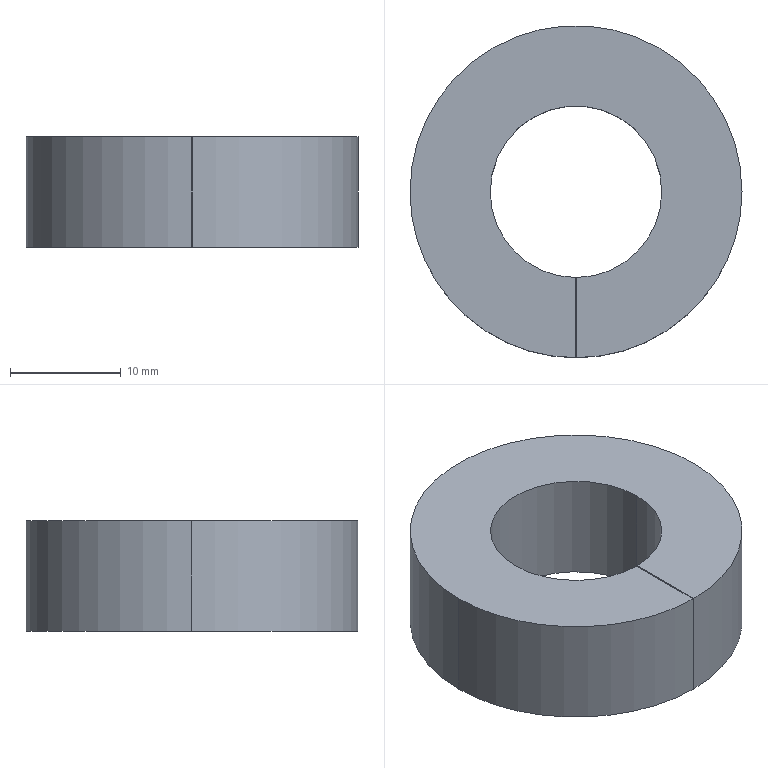Part | SolidWorks | features Extrusion 1, ICE 1 | 1 solid | 10 faces | box 30 x 30 x 10 mm | volume 5174 mm3 | cylinder 6 | plane 4 | commonest cylinder face diameters 15.5 x3 30 x3
STEP:
#1=CARTESIAN_POINT('',(0.05,-7.75,10.));
#2=VERTEX_POINT('',#1);
#3=CARTESIAN_POINT('',(7.75,0.,10.));
#4=VERTEX_POINT('',#3);
#5=CARTESIAN_POINT('',(0.,0.,10.));
#6=DIRECTION('',(0.,0.,1.));
#7=DIRECTION('',(1.,0.,0.));
#8=AXIS2_PLACEMENT_3D('',#5,#6,#7);
#9=CIRCLE('',#8,7.75);
#10=EDGE_CURVE('',#2,#4,#9,.T.);
#11=ORIENTED_EDGE('',*,*,#10,.T.);
#12=CARTESIAN_POINT('',(7.75,0.,0.));
#13=VERTEX_POINT('',#12);
#14=CARTESIAN_POINT('',(7.75,0.,10.));
#15=DIRECTION('',(0.,0.,-1.));
#16=VECTOR('',#15,1000.);
#17=LINE('',#14,#16);
#18=EDGE_CURVE('',#4,#13,#17,.T.);
#19=ORIENTED_EDGE('',*,*,#18,.T.);
#20=CARTESIAN_POINT('',(0.05,-7.75,0.));
#21=VERTEX_POINT('',#20);
#22=CARTESIAN_POINT('',(0.,0.,0.));
#23=DIRECTION('',(0.,0.,1.));
#24=DIRECTION('',(1.,0.,0.));
#25=AXIS2_PLACEMENT_3D('',#22,#23,#24);
#26=CIRCLE('',#25,7.75);
#27=EDGE_CURVE('',#21,#13,#26,.T.);
#28=ORIENTED_EDGE('',*,*,#27,.F.);
#29=CARTESIAN_POINT('',(0.05,-7.75,10.));
#30=DIRECTION('',(0.,0.,-1.));
#31=VECTOR('',#30,1000.);
#32=LINE('',#29,#31);
#33=EDGE_CURVE('',#2,#21,#32,.T.);
#34=ORIENTED_EDGE('',*,*,#33,.F.);
#35=EDGE_LOOP('',(#11,#19,#28,#34));
#36=FACE_OUTER_BOUND('',#35,.T.);
#37=CARTESIAN_POINT('',(0.,0.,10.));
#38=DIRECTION('',(0.,0.,-1.));
#39=DIRECTION('',(-1.,0.,0.));
#40=AXIS2_PLACEMENT_3D('',#37,#38,#39);
#41=CYLINDRICAL_SURFACE('',#40,7.75);
#42=ADVANCED_FACE('',(#36),#41,.F.);
#43=ORIENTED_EDGE('',*,*,#18,.F.);
#44=CARTESIAN_POINT('',(-7.75,0.,10.));
#45=VERTEX_POINT('',#44);
#46=CARTESIAN_POINT('',(0.,0.,10.));
#47=DIRECTION('',(0.,0.,1.));
#48=DIRECTION('',(1.,0.,0.));
#49=AXIS2_PLACEMENT_3D('',#46,#47,#48);
#50=CIRCLE('',#49,7.75);
#51=EDGE_CURVE('',#4,#45,#50,.T.);
#52=ORIENTED_EDGE('',*,*,#51,.T.);
#53=CARTESIAN_POINT('',(-7.75,0.,0.));
#54=VERTEX_POINT('',#53);
#55=CARTESIAN_POINT('',(-7.75,0.,10.));
#56=DIRECTION('',(0.,0.,-1.));
#57=VECTOR('',#56,1000.);
#58=LINE('',#55,#57);
#59=EDGE_CURVE('',#45,#54,#58,.T.);
#60=ORIENTED_EDGE('',*,*,#59,.T.);
#61=CARTESIAN_POINT('',(0.,0.,0.));
#62=DIRECTION('',(0.,0.,1.));
#63=DIRECTION('',(1.,0.,0.));
#64=AXIS2_PLACEMENT_3D('',#61,#62,#63);
#65=CIRCLE('',#64,7.75);
#66=EDGE_CURVE('',#13,#54,#65,.T.);
#67=ORIENTED_EDGE('',*,*,#66,.F.);
#68=EDGE_LOOP('',(#43,#52,#60,#67));
#69=FACE_OUTER_BOUND('',#68,.T.);
#70=CARTESIAN_POINT('',(0.,0.,10.));
#71=DIRECTION('',(0.,0.,-1.));
#72=DIRECTION('',(-1.,0.,0.));
#73=AXIS2_PLACEMENT_3D('',#70,#71,#72);
#74=CYLINDRICAL_SURFACE('',#73,7.75);
#75=ADVANCED_FACE('',(#69),#74,.F.);
#76=CARTESIAN_POINT('',(15.,0.,10.));
#77=VERTEX_POINT('',#76);
#78=CARTESIAN_POINT('',(-15.,0.,10.));
#79=VERTEX_POINT('',#78);
#80=CARTESIAN_POINT('',(0.,0.,10.));
#81=DIRECTION('',(0.,0.,1.));
#82=DIRECTION('',(1.,0.,0.));
#83=AXIS2_PLACEMENT_3D('',#80,#81,#82);
#84=CIRCLE('',#83,15.);
#85=EDGE_CURVE('',#77,#79,#84,.T.);
#86=ORIENTED_EDGE('',*,*,#85,.F.);
#87=CARTESIAN_POINT('',(15.,0.,0.));
#88=VERTEX_POINT('',#87);
#89=CARTESIAN_POINT('',(15.,0.,10.));
#90=DIRECTION('',(0.,0.,-1.));
#91=VECTOR('',#90,1000.);
#92=LINE('',#89,#91);
#93=EDGE_CURVE('',#77,#88,#92,.T.);
#94=ORIENTED_EDGE('',*,*,#93,.T.);
#95=CARTESIAN_POINT('',(-15.,0.,0.));
#96=VERTEX_POINT('',#95);
#97=CARTESIAN_POINT('',(0.,0.,0.));
#98=DIRECTION('',(0.,0.,1.));
#99=DIRECTION('',(1.,0.,0.));
#100=AXIS2_PLACEMENT_3D('',#97,#98,#99);
#101=CIRCLE('',#100,15.);
#102=EDGE_CURVE('',#88,#96,#101,.T.);
#103=ORIENTED_EDGE('',*,*,#102,.T.);
#104=CARTESIAN_POINT('',(-15.,0.,10.));
#105=DIRECTION('',(0.,0.,-1.));
#106=VECTOR('',#105,1000.);
#107=LINE('',#104,#106);
#108=EDGE_CURVE('',#79,#96,#107,.T.);
#109=ORIENTED_EDGE('',*,*,#108,.F.);
#110=EDGE_LOOP('',(#86,#94,#103,#109));
#111=FACE_OUTER_BOUND('',#110,.T.);
#112=CARTESIAN_POINT('',(0.,0.,10.));
#113=DIRECTION('',(0.,0.,-1.));
#114=DIRECTION('',(-1.,0.,0.));
#115=AXIS2_PLACEMENT_3D('',#112,#113,#114);
#116=CYLINDRICAL_SURFACE('',#115,15.);
#117=ADVANCED_FACE('',(#111),#116,.T.);
#118=CARTESIAN_POINT('',(-0.05,-15.,10.));
#119=VERTEX_POINT('',#118);
#120=CARTESIAN_POINT('',(0.,0.,10.));
#121=DIRECTION('',(0.,0.,1.));
#122=DIRECTION('',(1.,0.,0.));
#123=AXIS2_PLACEMENT_3D('',#120,#121,#122);
#124=CIRCLE('',#123,15.);
#125=EDGE_CURVE('',#79,#119,#124,.T.);
#126=ORIENTED_EDGE('',*,*,#125,.F.);
#127=ORIENTED_EDGE('',*,*,#108,.T.);
#128=CARTESIAN_POINT('',(-0.05,-15.,0.));
#129=VERTEX_POINT('',#128);
#130=CARTESIAN_POINT('',(0.,0.,0.));
#131=DIRECTION('',(0.,0.,1.));
#132=DIRECTION('',(1.,0.,0.));
#133=AXIS2_PLACEMENT_3D('',#130,#131,#132);
#134=CIRCLE('',#133,15.);
#135=EDGE_CURVE('',#96,#129,#134,.T.);
#136=ORIENTED_EDGE('',*,*,#135,.T.);
#137=CARTESIAN_POINT('',(-0.05,-15.,10.));
#138=DIRECTION('',(0.,0.,1.));
#139=VECTOR('',#138,1000.);
#140=LINE('',#137,#139);
#141=EDGE_CURVE('',#129,#119,#140,.T.);
#142=ORIENTED_EDGE('',*,*,#141,.T.);
#143=EDGE_LOOP('',(#126,#127,#136,#142));
#144=FACE_OUTER_BOUND('',#143,.T.);
#145=CARTESIAN_POINT('',(0.,0.,10.));
#146=DIRECTION('',(0.,0.,-1.));
#147=DIRECTION('',(-1.,0.,0.));
#148=AXIS2_PLACEMENT_3D('',#145,#146,#147);
#149=CYLINDRICAL_SURFACE('',#148,15.);
#150=ADVANCED_FACE('',(#144),#149,.T.);
#151=CARTESIAN_POINT('',(0.05,-15.,10.));
#152=VERTEX_POINT('',#151);
#153=CARTESIAN_POINT('',(0.05,3.484,10.));
#154=DIRECTION('',(0.,1.,0.));
#155=VECTOR('',#154,1000.);
#156=LINE('',#153,#155);
#157=EDGE_CURVE('',#152,#2,#156,.T.);
#158=ORIENTED_EDGE('',*,*,#157,.F.);
#159=CARTESIAN_POINT('',(0.,0.,10.));
#160=DIRECTION('',(0.,0.,1.));
#161=DIRECTION('',(1.,0.,0.));
#162=AXIS2_PLACEMENT_3D('',#159,#160,#161);
#163=CIRCLE('',#162,15.);
#164=EDGE_CURVE('',#152,#77,#163,.T.);
#165=ORIENTED_EDGE('',*,*,#164,.T.);
#166=ORIENTED_EDGE('',*,*,#85,.T.);
#167=ORIENTED_EDGE('',*,*,#125,.T.);
#168=CARTESIAN_POINT('',(-0.05,-7.75,10.));
#169=VERTEX_POINT('',#168);
#170=CARTESIAN_POINT('',(-0.05,3.484,10.));
#171=DIRECTION('',(0.,-1.,0.));
#172=VECTOR('',#171,1000.);
#173=LINE('',#170,#172);
#174=EDGE_CURVE('',#169,#119,#173,.T.);
#175=ORIENTED_EDGE('',*,*,#174,.F.);
#176=CARTESIAN_POINT('',(0.,0.,10.));
#177=DIRECTION('',(0.,0.,1.));
#178=DIRECTION('',(1.,0.,0.));
#179=AXIS2_PLACEMENT_3D('',#176,#177,#178);
#180=CIRCLE('',#179,7.75);
#181=EDGE_CURVE('',#45,#169,#180,.T.);
#182=ORIENTED_EDGE('',*,*,#181,.F.);
#183=ORIENTED_EDGE('',*,*,#51,.F.);
#184=ORIENTED_EDGE('',*,*,#10,.F.);
#185=EDGE_LOOP('',(#158,#165,#166,#167,#175,#182,#183,#184));
#186=FACE_OUTER_BOUND('',#185,.T.);
#187=CARTESIAN_POINT('',(0.,0.,10.));
#188=DIRECTION('',(0.,0.,1.));
#189=DIRECTION('',(1.,0.,0.));
#190=AXIS2_PLACEMENT_3D('',#187,#188,#189);
#191=PLANE('',#190);
#192=ADVANCED_FACE('',(#186),#191,.T.);
#193=CARTESIAN_POINT('',(0.05,-15.,0.));
#194=VERTEX_POINT('',#193);
#195=CARTESIAN_POINT('',(0.,0.,0.));
#196=DIRECTION('',(0.,0.,1.));
#197=DIRECTION('',(1.,0.,0.));
#198=AXIS2_PLACEMENT_3D('',#195,#196,#197);
#199=CIRCLE('',#198,15.);
#200=EDGE_CURVE('',#194,#88,#199,.T.);
#201=ORIENTED_EDGE('',*,*,#200,.F.);
#202=CARTESIAN_POINT('',(0.05,3.484,0.));
#203=DIRECTION('',(0.,1.,0.));
#204=VECTOR('',#203,1000.);
#205=LINE('',#202,#204);
#206=EDGE_CURVE('',#194,#21,#205,.T.);
#207=ORIENTED_EDGE('',*,*,#206,.T.);
#208=ORIENTED_EDGE('',*,*,#27,.T.);
#209=ORIENTED_EDGE('',*,*,#66,.T.);
#210=CARTESIAN_POINT('',(-0.05,-7.75,0.));
#211=VERTEX_POINT('',#210);
#212=CARTESIAN_POINT('',(0.,0.,0.));
#213=DIRECTION('',(0.,0.,1.));
#214=DIRECTION('',(1.,0.,0.));
#215=AXIS2_PLACEMENT_3D('',#212,#213,#214);
#216=CIRCLE('',#215,7.75);
#217=EDGE_CURVE('',#54,#211,#216,.T.);
#218=ORIENTED_EDGE('',*,*,#217,.T.);
#219=CARTESIAN_POINT('',(-0.05,3.484,0.));
#220=DIRECTION('',(0.,-1.,0.));
#221=VECTOR('',#220,1000.);
#222=LINE('',#219,#221);
#223=EDGE_CURVE('',#211,#129,#222,.T.);
#224=ORIENTED_EDGE('',*,*,#223,.T.);
#225=ORIENTED_EDGE('',*,*,#135,.F.);
#226=ORIENTED_EDGE('',*,*,#102,.F.);
#227=EDGE_LOOP('',(#201,#207,#208,#209,#218,#224,#225,#226));
#228=FACE_OUTER_BOUND('',#227,.T.);
#229=CARTESIAN_POINT('',(0.,0.,0.));
#230=DIRECTION('',(0.,0.,1.));
#231=DIRECTION('',(1.,0.,0.));
#232=AXIS2_PLACEMENT_3D('',#229,#230,#231);
#233=PLANE('',#232);
#234=ADVANCED_FACE('',(#228),#233,.F.);
#235=ORIENTED_EDGE('',*,*,#93,.F.);
#236=ORIENTED_EDGE('',*,*,#164,.F.);
#237=CARTESIAN_POINT('',(0.05,-15.,10.));
#238=DIRECTION('',(0.,0.,-1.));
#239=VECTOR('',#238,1000.);
#240=LINE('',#237,#239);
#241=EDGE_CURVE('',#152,#194,#240,.T.);
#242=ORIENTED_EDGE('',*,*,#241,.T.);
#243=ORIENTED_EDGE('',*,*,#200,.T.);
#244=EDGE_LOOP('',(#235,#236,#242,#243));
#245=FACE_OUTER_BOUND('',#244,.T.);
#246=CARTESIAN_POINT('',(0.,0.,10.));
#247=DIRECTION('',(0.,0.,-1.));
#248=DIRECTION('',(-1.,0.,0.));
#249=AXIS2_PLACEMENT_3D('',#246,#247,#248);
#250=CYLINDRICAL_SURFACE('',#249,15.);
#251=ADVANCED_FACE('',(#245),#250,.T.);
#252=ORIENTED_EDGE('',*,*,#59,.F.);
#253=ORIENTED_EDGE('',*,*,#181,.T.);
#254=CARTESIAN_POINT('',(-0.05,-7.75,10.));
#255=DIRECTION('',(0.,0.,1.));
#256=VECTOR('',#255,1000.);
#257=LINE('',#254,#256);
#258=EDGE_CURVE('',#211,#169,#257,.T.);
#259=ORIENTED_EDGE('',*,*,#258,.F.);
#260=ORIENTED_EDGE('',*,*,#217,.F.);
#261=EDGE_LOOP('',(#252,#253,#259,#260));
#262=FACE_OUTER_BOUND('',#261,.T.);
#263=CARTESIAN_POINT('',(0.,0.,10.));
#264=DIRECTION('',(0.,0.,-1.));
#265=DIRECTION('',(-1.,0.,0.));
#266=AXIS2_PLACEMENT_3D('',#263,#264,#265);
#267=CYLINDRICAL_SURFACE('',#266,7.75);
#268=ADVANCED_FACE('',(#262),#267,.F.);
#269=ORIENTED_EDGE('',*,*,#223,.F.);
#270=ORIENTED_EDGE('',*,*,#258,.T.);
#271=ORIENTED_EDGE('',*,*,#174,.T.);
#272=ORIENTED_EDGE('',*,*,#141,.F.);
#273=EDGE_LOOP('',(#269,#270,#271,#272));
#274=FACE_OUTER_BOUND('',#273,.T.);
#275=CARTESIAN_POINT('',(-0.05,3.484,0.));
#276=DIRECTION('',(-1.,0.,0.));
#277=DIRECTION('',(0.,-1.,0.));
#278=AXIS2_PLACEMENT_3D('',#275,#276,#277);
#279=PLANE('',#278);
#280=ADVANCED_FACE('',(#274),#279,.F.);
#281=ORIENTED_EDGE('',*,*,#157,.T.);
#282=ORIENTED_EDGE('',*,*,#33,.T.);
#283=ORIENTED_EDGE('',*,*,#206,.F.);
#284=ORIENTED_EDGE('',*,*,#241,.F.);
#285=EDGE_LOOP('',(#281,#282,#283,#284));
#286=FACE_OUTER_BOUND('',#285,.T.);
#287=CARTESIAN_POINT('',(0.05,3.484,0.));
#288=DIRECTION('',(1.,0.,0.));
#289=DIRECTION('',(0.,1.,0.));
#290=AXIS2_PLACEMENT_3D('',#287,#288,#289);
#291=PLANE('',#290);
#292=ADVANCED_FACE('',(#286),#291,.F.);
#293=CLOSED_SHELL('',(#42,#75,#117,#150,#192,#234,#251,#268,#280,#292));
#294=MANIFOLD_SOLID_BREP('',#293);
#295=CARTESIAN_POINT('',(0.,0.,0.));
#296=DIRECTION('',(0.,0.,1.));
#297=DIRECTION('',(1.,0.,0.));
#298=AXIS2_PLACEMENT_3D('',#295,#296,#297);
#299=(LENGTH_UNIT()NAMED_UNIT(*)SI_UNIT(.MILLI.,.METRE.));
#300=UNCERTAINTY_MEASURE_WITH_UNIT(LENGTH_MEASURE(0.00001),#299,'','');
#301=(NAMED_UNIT(*)PLANE_ANGLE_UNIT()SI_UNIT($,.RADIAN.));
#302=(NAMED_UNIT(*)SI_UNIT($,.STERADIAN.)SOLID_ANGLE_UNIT());
#303=(GEOMETRIC_REPRESENTATION_CONTEXT(3)GLOBAL_UNCERTAINTY_ASSIGNED_CONTEXT((#300))GLOBAL_UNIT_ASSIGNED_CONTEXT((#299,#301,#302))REPRESENTATION_CONTEXT('',''));
#304=ADVANCED_BREP_SHAPE_REPRESENTATION('',(#294,#298),#303);